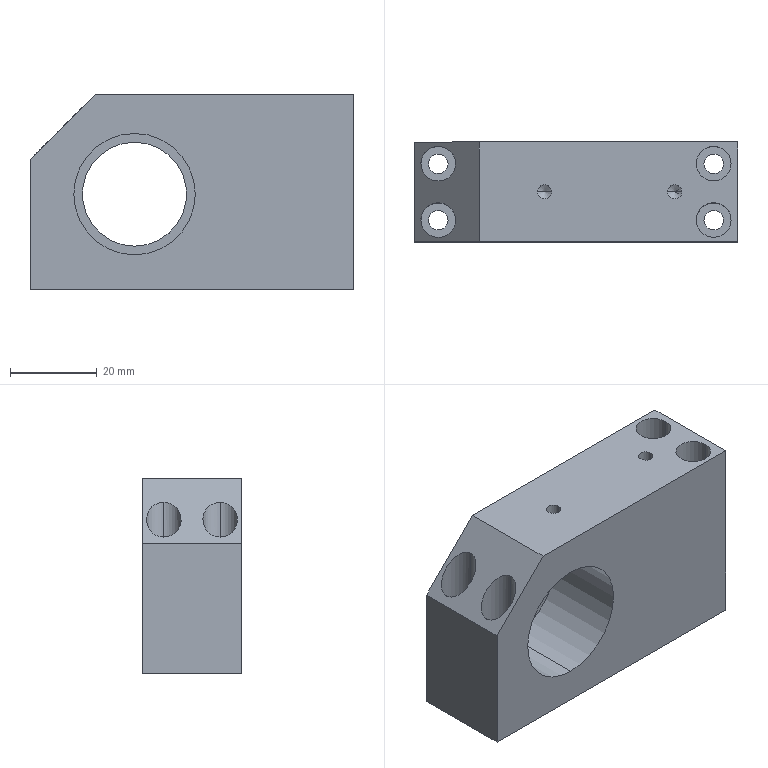Part | SolidWorks | features BaseBody 1 | 1 solid | 40 faces | box 74.5 x 23 x 45 mm | volume 54150 mm3 | cylinder 24 | plane 12 | cone 4 | commonest cylinder face diameters 4.5 x8 8 x8 3.3 x4 24 x2 28 x2
STEP:
#1=CARTESIAN_POINT('',(-13.25,19.,-12.5));
#2=VERTEX_POINT('',#1);
#3=CARTESIAN_POINT('',(-13.25,19.,11.5));
#4=VERTEX_POINT('',#3);
#5=CARTESIAN_POINT('',(-13.25,19.,-0.5));
#6=DIRECTION('',(0.,1.,0.));
#7=DIRECTION('',(0.,0.,1.));
#8=AXIS2_PLACEMENT_3D('',#5,#6,#7);
#9=CIRCLE('',#8,12.);
#10=EDGE_CURVE('',#2,#4,#9,.T.);
#11=ORIENTED_EDGE('',*,*,#10,.F.);
#12=CARTESIAN_POINT('',(-13.25,23.,-12.5));
#13=VERTEX_POINT('',#12);
#14=CARTESIAN_POINT('',(-13.25,-88.,-12.5));
#15=DIRECTION('',(0.,1.,0.));
#16=VECTOR('',#15,1000.);
#17=LINE('',#14,#16);
#18=EDGE_CURVE('',#2,#13,#17,.T.);
#19=ORIENTED_EDGE('',*,*,#18,.T.);
#20=CARTESIAN_POINT('',(-13.25,23.,11.5));
#21=VERTEX_POINT('',#20);
#22=CARTESIAN_POINT('',(-13.25,23.,-0.5));
#23=DIRECTION('',(0.,-1.,0.));
#24=DIRECTION('',(0.,0.,1.));
#25=AXIS2_PLACEMENT_3D('',#22,#23,#24);
#26=CIRCLE('',#25,12.);
#27=EDGE_CURVE('',#21,#13,#26,.T.);
#28=ORIENTED_EDGE('',*,*,#27,.F.);
#29=CARTESIAN_POINT('',(-13.25,-88.,11.5));
#30=DIRECTION('',(0.,1.,0.));
#31=VECTOR('',#30,1000.);
#32=LINE('',#29,#31);
#33=EDGE_CURVE('',#4,#21,#32,.T.);
#34=ORIENTED_EDGE('',*,*,#33,.F.);
#35=EDGE_LOOP('',(#11,#19,#28,#34));
#36=FACE_OUTER_BOUND('',#35,.T.);
#37=CARTESIAN_POINT('',(-13.25,-88.,-0.5));
#38=DIRECTION('',(0.,1.,0.));
#39=DIRECTION('',(0.,0.,1.));
#40=AXIS2_PLACEMENT_3D('',#37,#38,#39);
#41=CYLINDRICAL_SURFACE('',#40,12.);
#42=ADVANCED_FACE('',(#36),#41,.F.);
#43=CARTESIAN_POINT('',(-29.5,5.,-22.5));
#44=VERTEX_POINT('',#43);
#45=CARTESIAN_POINT('',(-34.,5.,-22.5));
#46=VERTEX_POINT('',#45);
#47=CARTESIAN_POINT('',(-31.75,5.,-22.5));
#48=DIRECTION('',(0.,0.,-1.));
#49=DIRECTION('',(1.,0.,0.));
#50=AXIS2_PLACEMENT_3D('',#47,#48,#49);
#51=CIRCLE('',#50,2.25);
#52=EDGE_CURVE('',#44,#46,#51,.T.);
#53=ORIENTED_EDGE('',*,*,#52,.T.);
#54=CARTESIAN_POINT('',(-34.,5.,-12.5));
#55=VERTEX_POINT('',#54);
#56=CARTESIAN_POINT('',(-34.,5.,22.5));
#57=DIRECTION('',(0.,0.,1.));
#58=VECTOR('',#57,1000.);
#59=LINE('',#56,#58);
#60=EDGE_CURVE('',#46,#55,#59,.T.);
#61=ORIENTED_EDGE('',*,*,#60,.T.);
#62=CARTESIAN_POINT('',(-29.5,5.,-12.5));
#63=VERTEX_POINT('',#62);
#64=CARTESIAN_POINT('',(-31.75,5.,-12.5));
#65=DIRECTION('',(0.,0.,-1.));
#66=DIRECTION('',(1.,0.,0.));
#67=AXIS2_PLACEMENT_3D('',#64,#65,#66);
#68=CIRCLE('',#67,2.25);
#69=EDGE_CURVE('',#63,#55,#68,.T.);
#70=ORIENTED_EDGE('',*,*,#69,.F.);
#71=CARTESIAN_POINT('',(-29.5,5.,22.5));
#72=DIRECTION('',(0.,0.,1.));
#73=VECTOR('',#72,1000.);
#74=LINE('',#71,#73);
#75=EDGE_CURVE('',#44,#63,#74,.T.);
#76=ORIENTED_EDGE('',*,*,#75,.F.);
#77=EDGE_LOOP('',(#53,#61,#70,#76));
#78=FACE_OUTER_BOUND('',#77,.T.);
#79=CARTESIAN_POINT('',(-31.75,5.,22.5));
#80=DIRECTION('',(0.,0.,1.));
#81=DIRECTION('',(1.,0.,0.));
#82=AXIS2_PLACEMENT_3D('',#79,#80,#81);
#83=CYLINDRICAL_SURFACE('',#82,2.25);
#84=ADVANCED_FACE('',(#78),#83,.F.);
#85=CARTESIAN_POINT('',(34.,5.,-22.5));
#86=VERTEX_POINT('',#85);
#87=CARTESIAN_POINT('',(29.5,5.,-22.5));
#88=VERTEX_POINT('',#87);
#89=CARTESIAN_POINT('',(31.75,5.,-22.5));
#90=DIRECTION('',(0.,0.,-1.));
#91=DIRECTION('',(1.,0.,0.));
#92=AXIS2_PLACEMENT_3D('',#89,#90,#91);
#93=CIRCLE('',#92,2.25);
#94=EDGE_CURVE('',#86,#88,#93,.T.);
#95=ORIENTED_EDGE('',*,*,#94,.T.);
#96=CARTESIAN_POINT('',(29.5,5.,-12.5));
#97=VERTEX_POINT('',#96);
#98=CARTESIAN_POINT('',(29.5,5.,22.5));
#99=DIRECTION('',(0.,0.,1.));
#100=VECTOR('',#99,1000.);
#101=LINE('',#98,#100);
#102=EDGE_CURVE('',#88,#97,#101,.T.);
#103=ORIENTED_EDGE('',*,*,#102,.T.);
#104=CARTESIAN_POINT('',(34.,5.,-12.5));
#105=VERTEX_POINT('',#104);
#106=CARTESIAN_POINT('',(31.75,5.,-12.5));
#107=DIRECTION('',(0.,0.,-1.));
#108=DIRECTION('',(1.,0.,0.));
#109=AXIS2_PLACEMENT_3D('',#106,#107,#108);
#110=CIRCLE('',#109,2.25);
#111=EDGE_CURVE('',#105,#97,#110,.T.);
#112=ORIENTED_EDGE('',*,*,#111,.F.);
#113=CARTESIAN_POINT('',(34.,5.,22.5));
#114=DIRECTION('',(0.,0.,1.));
#115=VECTOR('',#114,1000.);
#116=LINE('',#113,#115);
#117=EDGE_CURVE('',#86,#105,#116,.T.);
#118=ORIENTED_EDGE('',*,*,#117,.F.);
#119=EDGE_LOOP('',(#95,#103,#112,#118));
#120=FACE_OUTER_BOUND('',#119,.T.);
#121=CARTESIAN_POINT('',(31.75,5.,22.5));
#122=DIRECTION('',(0.,0.,1.));
#123=DIRECTION('',(1.,0.,0.));
#124=AXIS2_PLACEMENT_3D('',#121,#122,#123);
#125=CYLINDRICAL_SURFACE('',#124,2.25);
#126=ADVANCED_FACE('',(#120),#125,.F.);
#127=CARTESIAN_POINT('',(-29.5,18.,-22.5));
#128=VERTEX_POINT('',#127);
#129=CARTESIAN_POINT('',(-34.,18.,-22.5));
#130=VERTEX_POINT('',#129);
#131=CARTESIAN_POINT('',(-31.75,18.,-22.5));
#132=DIRECTION('',(0.,0.,-1.));
#133=DIRECTION('',(1.,0.,0.));
#134=AXIS2_PLACEMENT_3D('',#131,#132,#133);
#135=CIRCLE('',#134,2.25);
#136=EDGE_CURVE('',#128,#130,#135,.T.);
#137=ORIENTED_EDGE('',*,*,#136,.T.);
#138=CARTESIAN_POINT('',(-34.,18.,-12.5));
#139=VERTEX_POINT('',#138);
#140=CARTESIAN_POINT('',(-34.,18.,22.5));
#141=DIRECTION('',(0.,0.,1.));
#142=VECTOR('',#141,1000.);
#143=LINE('',#140,#142);
#144=EDGE_CURVE('',#130,#139,#143,.T.);
#145=ORIENTED_EDGE('',*,*,#144,.T.);
#146=CARTESIAN_POINT('',(-29.5,18.,-12.5));
#147=VERTEX_POINT('',#146);
#148=CARTESIAN_POINT('',(-31.75,18.,-12.5));
#149=DIRECTION('',(0.,0.,-1.));
#150=DIRECTION('',(1.,0.,0.));
#151=AXIS2_PLACEMENT_3D('',#148,#149,#150);
#152=CIRCLE('',#151,2.25);
#153=EDGE_CURVE('',#147,#139,#152,.T.);
#154=ORIENTED_EDGE('',*,*,#153,.F.);
#155=CARTESIAN_POINT('',(-29.5,18.,22.5));
#156=DIRECTION('',(0.,0.,1.));
#157=VECTOR('',#156,1000.);
#158=LINE('',#155,#157);
#159=EDGE_CURVE('',#128,#147,#158,.T.);
#160=ORIENTED_EDGE('',*,*,#159,.F.);
#161=EDGE_LOOP('',(#137,#145,#154,#160));
#162=FACE_OUTER_BOUND('',#161,.T.);
#163=CARTESIAN_POINT('',(-31.75,18.,22.5));
#164=DIRECTION('',(0.,0.,1.));
#165=DIRECTION('',(1.,0.,0.));
#166=AXIS2_PLACEMENT_3D('',#163,#164,#165);
#167=CYLINDRICAL_SURFACE('',#166,2.25);
#168=ADVANCED_FACE('',(#162),#167,.F.);
#169=CARTESIAN_POINT('',(34.,18.,-22.5));
#170=VERTEX_POINT('',#169);
#171=CARTESIAN_POINT('',(29.5,18.,-22.5));
#172=VERTEX_POINT('',#171);
#173=CARTESIAN_POINT('',(31.75,18.,-22.5));
#174=DIRECTION('',(0.,0.,-1.));
#175=DIRECTION('',(1.,0.,0.));
#176=AXIS2_PLACEMENT_3D('',#173,#174,#175);
#177=CIRCLE('',#176,2.25);
#178=EDGE_CURVE('',#170,#172,#177,.T.);
#179=ORIENTED_EDGE('',*,*,#178,.T.);
#180=CARTESIAN_POINT('',(29.5,18.,-12.5));
#181=VERTEX_POINT('',#180);
#182=CARTESIAN_POINT('',(29.5,18.,22.5));
#183=DIRECTION('',(0.,0.,1.));
#184=VECTOR('',#183,1000.);
#185=LINE('',#182,#184);
#186=EDGE_CURVE('',#172,#181,#185,.T.);
#187=ORIENTED_EDGE('',*,*,#186,.T.);
#188=CARTESIAN_POINT('',(34.,18.,-12.5));
#189=VERTEX_POINT('',#188);
#190=CARTESIAN_POINT('',(31.75,18.,-12.5));
#191=DIRECTION('',(0.,0.,-1.));
#192=DIRECTION('',(1.,0.,0.));
#193=AXIS2_PLACEMENT_3D('',#190,#191,#192);
#194=CIRCLE('',#193,2.25);
#195=EDGE_CURVE('',#189,#181,#194,.T.);
#196=ORIENTED_EDGE('',*,*,#195,.F.);
#197=CARTESIAN_POINT('',(34.,18.,22.5));
#198=DIRECTION('',(0.,0.,1.));
#199=VECTOR('',#198,1000.);
#200=LINE('',#197,#199);
#201=EDGE_CURVE('',#170,#189,#200,.T.);
#202=ORIENTED_EDGE('',*,*,#201,.F.);
#203=EDGE_LOOP('',(#179,#187,#196,#202));
#204=FACE_OUTER_BOUND('',#203,.T.);
#205=CARTESIAN_POINT('',(31.75,18.,22.5));
#206=DIRECTION('',(0.,0.,1.));
#207=DIRECTION('',(1.,0.,0.));
#208=AXIS2_PLACEMENT_3D('',#205,#206,#207);
#209=CYLINDRICAL_SURFACE('',#208,2.25);
#210=ADVANCED_FACE('',(#204),#209,.F.);
#211=CARTESIAN_POINT('',(27.75,5.,-12.5));
#212=VERTEX_POINT('',#211);
#213=CARTESIAN_POINT('',(35.75,5.,-12.5));
#214=VERTEX_POINT('',#213);
#215=CARTESIAN_POINT('',(31.75,5.,-12.5));
#216=DIRECTION('',(0.,0.,1.));
#217=DIRECTION('',(1.,0.,0.));
#218=AXIS2_PLACEMENT_3D('',#215,#216,#217);
#219=CIRCLE('',#218,4.);
#220=EDGE_CURVE('',#212,#214,#219,.T.);
#221=ORIENTED_EDGE('',*,*,#220,.F.);
#222=CARTESIAN_POINT('',(27.75,5.,22.5));
#223=VERTEX_POINT('',#222);
#224=CARTESIAN_POINT('',(27.75,5.,22.5));
#225=DIRECTION('',(0.,0.,1.));
#226=VECTOR('',#225,1000.);
#227=LINE('',#224,#226);
#228=EDGE_CURVE('',#212,#223,#227,.T.);
#229=ORIENTED_EDGE('',*,*,#228,.T.);
#230=CARTESIAN_POINT('',(35.75,5.,22.5));
#231=VERTEX_POINT('',#230);
#232=CARTESIAN_POINT('',(31.75,5.,22.5));
#233=DIRECTION('',(0.,0.,1.));
#234=DIRECTION('',(1.,0.,0.));
#235=AXIS2_PLACEMENT_3D('',#232,#233,#234);
#236=CIRCLE('',#235,4.);
#237=EDGE_CURVE('',#223,#231,#236,.T.);
#238=ORIENTED_EDGE('',*,*,#237,.T.);
#239=CARTESIAN_POINT('',(35.75,5.,22.5));
#240=DIRECTION('',(0.,0.,1.));
#241=VECTOR('',#240,1000.);
#242=LINE('',#239,#241);
#243=EDGE_CURVE('',#214,#231,#242,.T.);
#244=ORIENTED_EDGE('',*,*,#243,.F.);
#245=EDGE_LOOP('',(#221,#229,#238,#244));
#246=FACE_OUTER_BOUND('',#245,.T.);
#247=CARTESIAN_POINT('',(31.75,5.,22.5));
#248=DIRECTION('',(0.,0.,1.));
#249=DIRECTION('',(1.,0.,0.));
#250=AXIS2_PLACEMENT_3D('',#247,#248,#249);
#251=CYLINDRICAL_SURFACE('',#250,4.);
#252=ADVANCED_FACE('',(#246),#251,.F.);
#253=CARTESIAN_POINT('',(27.75,18.,-12.5));
#254=VERTEX_POINT('',#253);
#255=CARTESIAN_POINT('',(35.75,18.,-12.5));
#256=VERTEX_POINT('',#255);
#257=CARTESIAN_POINT('',(31.75,18.,-12.5));
#258=DIRECTION('',(0.,0.,1.));
#259=DIRECTION('',(1.,0.,0.));
#260=AXIS2_PLACEMENT_3D('',#257,#258,#259);
#261=CIRCLE('',#260,4.);
#262=EDGE_CURVE('',#254,#256,#261,.T.);
#263=ORIENTED_EDGE('',*,*,#262,.F.);
#264=CARTESIAN_POINT('',(27.75,18.,22.5));
#265=VERTEX_POINT('',#264);
#266=CARTESIAN_POINT('',(27.75,18.,22.5));
#267=DIRECTION('',(0.,0.,1.));
#268=VECTOR('',#267,1000.);
#269=LINE('',#266,#268);
#270=EDGE_CURVE('',#254,#265,#269,.T.);
#271=ORIENTED_EDGE('',*,*,#270,.T.);
#272=CARTESIAN_POINT('',(35.75,18.,22.5));
#273=VERTEX_POINT('',#272);
#274=CARTESIAN_POINT('',(31.75,18.,22.5));
#275=DIRECTION('',(0.,0.,1.));
#276=DIRECTION('',(1.,0.,0.));
#277=AXIS2_PLACEMENT_3D('',#274,#275,#276);
#278=CIRCLE('',#277,4.);
#279=EDGE_CURVE('',#265,#273,#278,.T.);
#280=ORIENTED_EDGE('',*,*,#279,.T.);
#281=CARTESIAN_POINT('',(35.75,18.,22.5));
#282=DIRECTION('',(0.,0.,1.));
#283=VECTOR('',#282,1000.);
#284=LINE('',#281,#283);
#285=EDGE_CURVE('',#256,#273,#284,.T.);
#286=ORIENTED_EDGE('',*,*,#285,.F.);
#287=EDGE_LOOP('',(#263,#271,#280,#286));
#288=FACE_OUTER_BOUND('',#287,.T.);
#289=CARTESIAN_POINT('',(31.75,18.,22.5));
#290=DIRECTION('',(0.,0.,1.));
#291=DIRECTION('',(1.,0.,0.));
#292=AXIS2_PLACEMENT_3D('',#289,#290,#291);
#293=CYLINDRICAL_SURFACE('',#292,4.);
#294=ADVANCED_FACE('',(#288),#293,.F.);
#295=CARTESIAN_POINT('',(-8.9,11.5,14.5));
#296=VERTEX_POINT('',#295);
#297=CARTESIAN_POINT('',(-5.6,11.5,14.5));
#298=VERTEX_POINT('',#297);
#299=CARTESIAN_POINT('',(-7.25,11.5,14.5));
#300=DIRECTION('',(0.,0.,1.));
#301=DIRECTION('',(1.,0.,0.));
#302=AXIS2_PLACEMENT_3D('',#299,#300,#301);
#303=CIRCLE('',#302,1.65);
#304=EDGE_CURVE('',#296,#298,#303,.T.);
#305=ORIENTED_EDGE('',*,*,#304,.F.);
#306=CARTESIAN_POINT('',(-8.9,11.5,22.5));
#307=VERTEX_POINT('',#306);
#308=CARTESIAN_POINT('',(-8.9,11.5,22.5));
#309=DIRECTION('',(0.,0.,1.));
#310=VECTOR('',#309,1000.);
#311=LINE('',#308,#310);
#312=EDGE_CURVE('',#296,#307,#311,.T.);
#313=ORIENTED_EDGE('',*,*,#312,.T.);
#314=CARTESIAN_POINT('',(-5.6,11.5,22.5));
#315=VERTEX_POINT('',#314);
#316=CARTESIAN_POINT('',(-7.25,11.5,22.5));
#317=DIRECTION('',(0.,0.,1.));
#318=DIRECTION('',(1.,0.,0.));
#319=AXIS2_PLACEMENT_3D('',#316,#317,#318);
#320=CIRCLE('',#319,1.65);
#321=EDGE_CURVE('',#307,#315,#320,.T.);
#322=ORIENTED_EDGE('',*,*,#321,.T.);
#323=CARTESIAN_POINT('',(-5.6,11.5,22.5));
#324=DIRECTION('',(0.,0.,1.));
#325=VECTOR('',#324,1000.);
#326=LINE('',#323,#325);
#327=EDGE_CURVE('',#298,#315,#326,.T.);
#328=ORIENTED_EDGE('',*,*,#327,.F.);
#329=EDGE_LOOP('',(#305,#313,#322,#328));
#330=FACE_OUTER_BOUND('',#329,.T.);
#331=CARTESIAN_POINT('',(-7.25,11.5,22.5));
#332=DIRECTION('',(0.,0.,1.));
#333=DIRECTION('',(1.,0.,0.));
#334=AXIS2_PLACEMENT_3D('',#331,#332,#333);
#335=CYLINDRICAL_SURFACE('',#334,1.65);
#336=ADVANCED_FACE('',(#330),#335,.F.);
#337=CARTESIAN_POINT('',(21.1,11.5,14.5));
#338=VERTEX_POINT('',#337);
#339=CARTESIAN_POINT('',(24.4,11.5,14.5));
#340=VERTEX_POINT('',#339);
#341=CARTESIAN_POINT('',(22.75,11.5,14.5));
#342=DIRECTION('',(0.,0.,1.));
#343=DIRECTION('',(1.,0.,0.));
#344=AXIS2_PLACEMENT_3D('',#341,#342,#343);
#345=CIRCLE('',#344,1.65);
#346=EDGE_CURVE('',#338,#340,#345,.T.);
#347=ORIENTED_EDGE('',*,*,#346,.F.);
#348=CARTESIAN_POINT('',(21.1,11.5,22.5));
#349=VERTEX_POINT('',#348);
#350=CARTESIAN_POINT('',(21.1,11.5,22.5));
#351=DIRECTION('',(0.,0.,1.));
#352=VECTOR('',#351,1000.);
#353=LINE('',#350,#352);
#354=EDGE_CURVE('',#338,#349,#353,.T.);
#355=ORIENTED_EDGE('',*,*,#354,.T.);
#356=CARTESIAN_POINT('',(24.4,11.5,22.5));
#357=VERTEX_POINT('',#356);
#358=CARTESIAN_POINT('',(22.75,11.5,22.5));
#359=DIRECTION('',(0.,0.,1.));
#360=DIRECTION('',(1.,0.,0.));
#361=AXIS2_PLACEMENT_3D('',#358,#359,#360);
#362=CIRCLE('',#361,1.65);
#363=EDGE_CURVE('',#349,#357,#362,.T.);
#364=ORIENTED_EDGE('',*,*,#363,.T.);
#365=CARTESIAN_POINT('',(24.4,11.5,22.5));
#366=DIRECTION('',(0.,0.,1.));
#367=VECTOR('',#366,1000.);
#368=LINE('',#365,#367);
#369=EDGE_CURVE('',#340,#357,#368,.T.);
#370=ORIENTED_EDGE('',*,*,#369,.F.);
#371=EDGE_LOOP('',(#347,#355,#364,#370));
#372=FACE_OUTER_BOUND('',#371,.T.);
#373=CARTESIAN_POINT('',(22.75,11.5,22.5));
#374=DIRECTION('',(0.,0.,1.));
#375=DIRECTION('',(1.,0.,0.));
#376=AXIS2_PLACEMENT_3D('',#373,#374,#375);
#377=CYLINDRICAL_SURFACE('',#376,1.65);
#378=ADVANCED_FACE('',(#372),#377,.F.);
#379=CARTESIAN_POINT('',(-35.75,5.,-12.5));
#380=VERTEX_POINT('',#379);
#381=CARTESIAN_POINT('',(-27.75,5.,-12.5));
#382=VERTEX_POINT('',#381);
#383=CARTESIAN_POINT('',(-31.75,5.,-12.5));
#384=DIRECTION('',(0.,0.,1.));
#385=DIRECTION('',(1.,0.,0.));
#386=AXIS2_PLACEMENT_3D('',#383,#384,#385);
#387=CIRCLE('',#386,4.);
#388=EDGE_CURVE('',#380,#382,#387,.T.);
#389=ORIENTED_EDGE('',*,*,#388,.F.);
#390=CARTESIAN_POINT('',(-35.75,5.,9.));
#391=VERTEX_POINT('',#390);
#392=CARTESIAN_POINT('',(-35.75,5.,22.5));
#393=DIRECTION('',(0.,0.,1.));
#394=VECTOR('',#393,1000.);
#395=LINE('',#392,#394);
#396=EDGE_CURVE('',#380,#391,#395,.T.);
#397=ORIENTED_EDGE('',*,*,#396,.T.);
#398=CARTESIAN_POINT('',(-27.75,5.,17.));
#399=VERTEX_POINT('',#398);
#400=CARTESIAN_POINT('',(-35.75,5.,9.));
#401=CARTESIAN_POINT('',(-35.75,-3.,9.));
#402=CARTESIAN_POINT('',(-27.75,-3.,17.));
#403=CARTESIAN_POINT('',(-27.75,5.,17.));
#404=(BOUNDED_CURVE()B_SPLINE_CURVE(3,(#400,#401,#402,#403),.UNSPECIFIED.,.F.,.F.)B_SPLINE_CURVE_WITH_KNOTS((4,4),(3.142,6.283),.UNSPECIFIED.)CURVE()GEOMETRIC_REPRESENTATION_ITEM()RATIONAL_B_SPLINE_CURVE((1.,0.3333,0.3333,1.))REPRESENTATION_ITEM(''));
#405=EDGE_CURVE('',#391,#399,#404,.T.);
#406=ORIENTED_EDGE('',*,*,#405,.T.);
#407=CARTESIAN_POINT('',(-27.75,5.,22.5));
#408=DIRECTION('',(0.,0.,1.));
#409=VECTOR('',#408,1000.);
#410=LINE('',#407,#409);
#411=EDGE_CURVE('',#382,#399,#410,.T.);
#412=ORIENTED_EDGE('',*,*,#411,.F.);
#413=EDGE_LOOP('',(#389,#397,#406,#412));
#414=FACE_OUTER_BOUND('',#413,.T.);
#415=CARTESIAN_POINT('',(-31.75,5.,22.5));
#416=DIRECTION('',(0.,0.,1.));
#417=DIRECTION('',(1.,0.,0.));
#418=AXIS2_PLACEMENT_3D('',#415,#416,#417);
#419=CYLINDRICAL_SURFACE('',#418,4.);
#420=ADVANCED_FACE('',(#414),#419,.F.);
#421=CARTESIAN_POINT('',(-35.75,18.,-12.5));
#422=VERTEX_POINT('',#421);
#423=CARTESIAN_POINT('',(-27.75,18.,-12.5));
#424=VERTEX_POINT('',#423);
#425=CARTESIAN_POINT('',(-31.75,18.,-12.5));
#426=DIRECTION('',(0.,0.,1.));
#427=DIRECTION('',(1.,0.,0.));
#428=AXIS2_PLACEMENT_3D('',#425,#426,#427);
#429=CIRCLE('',#428,4.);
#430=EDGE_CURVE('',#422,#424,#429,.T.);
#431=ORIENTED_EDGE('',*,*,#430,.F.);
#432=CARTESIAN_POINT('',(-35.75,18.,9.));
#433=VERTEX_POINT('',#432);
#434=CARTESIAN_POINT('',(-35.75,18.,22.5));
#435=DIRECTION('',(0.,0.,1.));
#436=VECTOR('',#435,1000.);
#437=LINE('',#434,#436);
#438=EDGE_CURVE('',#422,#433,#437,.T.);
#439=ORIENTED_EDGE('',*,*,#438,.T.);
#440=CARTESIAN_POINT('',(-27.75,18.,17.));
#441=VERTEX_POINT('',#440);
#442=CARTESIAN_POINT('',(-35.75,18.,9.));
#443=CARTESIAN_POINT('',(-35.75,10.,9.));
#444=CARTESIAN_POINT('',(-27.75,10.,17.));
#445=CARTESIAN_POINT('',(-27.75,18.,17.));
#446=(BOUNDED_CURVE()B_SPLINE_CURVE(3,(#442,#443,#444,#445),.UNSPECIFIED.,.F.,.F.)B_SPLINE_CURVE_WITH_KNOTS((4,4),(3.142,6.283),.UNSPECIFIED.)CURVE()GEOMETRIC_REPRESENTATION_ITEM()RATIONAL_B_SPLINE_CURVE((1.,0.3333,0.3333,1.))REPRESENTATION_ITEM(''));
#447=EDGE_CURVE('',#433,#441,#446,.T.);
#448=ORIENTED_EDGE('',*,*,#447,.T.);
#449=CARTESIAN_POINT('',(-27.75,18.,22.5));
#450=DIRECTION('',(0.,0.,1.));
#451=VECTOR('',#450,1000.);
#452=LINE('',#449,#451);
#453=EDGE_CURVE('',#424,#441,#452,.T.);
#454=ORIENTED_EDGE('',*,*,#453,.F.);
#455=EDGE_LOOP('',(#431,#439,#448,#454));
#456=FACE_OUTER_BOUND('',#455,.T.);
#457=CARTESIAN_POINT('',(-31.75,18.,22.5));
#458=DIRECTION('',(0.,0.,1.));
#459=DIRECTION('',(1.,0.,0.));
#460=AXIS2_PLACEMENT_3D('',#457,#458,#459);
#461=CYLINDRICAL_SURFACE('',#460,4.);
#462=ADVANCED_FACE('',(#456),#461,.F.);
#463=CARTESIAN_POINT('',(-13.25,19.,13.5));
#464=VERTEX_POINT('',#463);
#465=CARTESIAN_POINT('',(-13.25,19.,-14.5));
#466=VERTEX_POINT('',#465);
#467=CARTESIAN_POINT('',(-13.25,19.,-0.5));
#468=DIRECTION('',(0.,-1.,0.));
#469=DIRECTION('',(0.,0.,-1.));
#470=AXIS2_PLACEMENT_3D('',#467,#468,#469);
#471=CIRCLE('',#470,14.);
#472=EDGE_CURVE('',#464,#466,#471,.T.);
#473=ORIENTED_EDGE('',*,*,#472,.F.);
#474=CARTESIAN_POINT('',(-13.25,0.,13.5));
#475=VERTEX_POINT('',#474);
#476=CARTESIAN_POINT('',(-13.25,19.,13.5));
#477=DIRECTION('',(0.,-1.,0.));
#478=VECTOR('',#477,1000.);
#479=LINE('',#476,#478);
#480=EDGE_CURVE('',#464,#475,#479,.T.);
#481=ORIENTED_EDGE('',*,*,#480,.T.);
#482=CARTESIAN_POINT('',(-13.25,0.,-14.5));
#483=VERTEX_POINT('',#482);
#484=CARTESIAN_POINT('',(-13.25,0.,-0.5));
#485=DIRECTION('',(0.,-1.,0.));
#486=DIRECTION('',(0.,0.,-1.));
#487=AXIS2_PLACEMENT_3D('',#484,#485,#486);
#488=CIRCLE('',#487,14.);
#489=EDGE_CURVE('',#475,#483,#488,.T.);
#490=ORIENTED_EDGE('',*,*,#489,.T.);
#491=CARTESIAN_POINT('',(-13.25,19.,-14.5));
#492=DIRECTION('',(0.,-1.,0.));
#493=VECTOR('',#492,1000.);
#494=LINE('',#491,#493);
#495=EDGE_CURVE('',#466,#483,#494,.T.);
#496=ORIENTED_EDGE('',*,*,#495,.F.);
#497=EDGE_LOOP('',(#473,#481,#490,#496));
#498=FACE_OUTER_BOUND('',#497,.T.);
#499=CARTESIAN_POINT('',(-13.25,19.,-0.5));
#500=DIRECTION('',(0.,-1.,0.));
#501=DIRECTION('',(0.,0.,-1.));
#502=AXIS2_PLACEMENT_3D('',#499,#500,#501);
#503=CYLINDRICAL_SURFACE('',#502,14.);
#504=ADVANCED_FACE('',(#498),#503,.F.);
#505=CARTESIAN_POINT('',(-7.25,11.5,13.509));
#506=VERTEX_POINT('',#505);
#507=CARTESIAN_POINT('',(-5.6,11.5,14.5));
#508=DIRECTION('',(0.8572,0.,0.515));
#509=VECTOR('',#508,1000.);
#510=LINE('',#507,#509);
#511=EDGE_CURVE('',#506,#298,#510,.T.);
#512=ORIENTED_EDGE('',*,*,#511,.F.);
#513=CARTESIAN_POINT('',(-8.9,11.5,14.5));
#514=DIRECTION('',(-0.8572,0.,0.515));
#515=VECTOR('',#514,1000.);
#516=LINE('',#513,#515);
#517=EDGE_CURVE('',#506,#296,#516,.T.);
#518=ORIENTED_EDGE('',*,*,#517,.T.);
#519=ORIENTED_EDGE('',*,*,#304,.T.);
#520=EDGE_LOOP('',(#512,#518,#519));
#521=FACE_OUTER_BOUND('',#520,.T.);
#522=CARTESIAN_POINT('',(-7.25,11.5,14.5));
#523=DIRECTION('',(0.,0.,1.));
#524=DIRECTION('',(1.,0.,0.));
#525=AXIS2_PLACEMENT_3D('',#522,#523,#524);
#526=CONICAL_SURFACE('',#525,1.65,1.03);
#527=ADVANCED_FACE('',(#521),#526,.F.);
#528=CARTESIAN_POINT('',(22.75,11.5,13.509));
#529=VERTEX_POINT('',#528);
#530=CARTESIAN_POINT('',(24.4,11.5,14.5));
#531=DIRECTION('',(0.8572,0.,0.515));
#532=VECTOR('',#531,1000.);
#533=LINE('',#530,#532);
#534=EDGE_CURVE('',#529,#340,#533,.T.);
#535=ORIENTED_EDGE('',*,*,#534,.F.);
#536=CARTESIAN_POINT('',(21.1,11.5,14.5));
#537=DIRECTION('',(-0.8572,0.,0.515));
#538=VECTOR('',#537,1000.);
#539=LINE('',#536,#538);
#540=EDGE_CURVE('',#529,#338,#539,.T.);
#541=ORIENTED_EDGE('',*,*,#540,.T.);
#542=ORIENTED_EDGE('',*,*,#346,.T.);
#543=EDGE_LOOP('',(#535,#541,#542));
#544=FACE_OUTER_BOUND('',#543,.T.);
#545=CARTESIAN_POINT('',(22.75,11.5,14.5));
#546=DIRECTION('',(0.,0.,1.));
#547=DIRECTION('',(1.,0.,0.));
#548=AXIS2_PLACEMENT_3D('',#545,#546,#547);
#549=CONICAL_SURFACE('',#548,1.65,1.03);
#550=ADVANCED_FACE('',(#544),#549,.F.);
#551=ORIENTED_EDGE('',*,*,#27,.T.);
#552=CARTESIAN_POINT('',(-13.25,23.,-0.5));
#553=DIRECTION('',(0.,-1.,0.));
#554=DIRECTION('',(0.,0.,1.));
#555=AXIS2_PLACEMENT_3D('',#552,#553,#554);
#556=CIRCLE('',#555,12.);
#557=EDGE_CURVE('',#13,#21,#556,.T.);
#558=ORIENTED_EDGE('',*,*,#557,.T.);
#559=EDGE_LOOP('',(#551,#558));
#560=FACE_BOUND('',#559,.T.);
#561=CARTESIAN_POINT('',(37.25,23.,-22.5));
#562=VERTEX_POINT('',#561);
#563=CARTESIAN_POINT('',(-37.25,23.,-22.5));
#564=VERTEX_POINT('',#563);
#565=CARTESIAN_POINT('',(0.,23.,-22.5));
#566=DIRECTION('',(-1.,0.,0.));
#567=VECTOR('',#566,1000.);
#568=LINE('',#565,#567);
#569=EDGE_CURVE('',#562,#564,#568,.T.);
#570=ORIENTED_EDGE('',*,*,#569,.T.);
#571=CARTESIAN_POINT('',(-37.25,23.,7.5));
#572=VERTEX_POINT('',#571);
#573=CARTESIAN_POINT('',(-37.25,23.,0.));
#574=DIRECTION('',(0.,0.,1.));
#575=VECTOR('',#574,1000.);
#576=LINE('',#573,#575);
#577=EDGE_CURVE('',#564,#572,#576,.T.);
#578=ORIENTED_EDGE('',*,*,#577,.T.);
#579=CARTESIAN_POINT('',(-22.25,23.,22.5));
#580=VERTEX_POINT('',#579);
#581=CARTESIAN_POINT('',(-37.25,23.,7.5));
#582=DIRECTION('',(0.7071,0.,0.7071));
#583=VECTOR('',#582,1000.);
#584=LINE('',#581,#583);
#585=EDGE_CURVE('',#572,#580,#584,.T.);
#586=ORIENTED_EDGE('',*,*,#585,.T.);
#587=CARTESIAN_POINT('',(37.25,23.,22.5));
#588=VERTEX_POINT('',#587);
#589=CARTESIAN_POINT('',(0.,23.,22.5));
#590=DIRECTION('',(1.,0.,0.));
#591=VECTOR('',#590,1000.);
#592=LINE('',#589,#591);
#593=EDGE_CURVE('',#580,#588,#592,.T.);
#594=ORIENTED_EDGE('',*,*,#593,.T.);
#595=CARTESIAN_POINT('',(37.25,23.,0.));
#596=DIRECTION('',(0.,0.,-1.));
#597=VECTOR('',#596,1000.);
#598=LINE('',#595,#597);
#599=EDGE_CURVE('',#588,#562,#598,.T.);
#600=ORIENTED_EDGE('',*,*,#599,.T.);
#601=EDGE_LOOP('',(#570,#578,#586,#594,#600));
#602=FACE_OUTER_BOUND('',#601,.T.);
#603=CARTESIAN_POINT('',(0.,23.,0.));
#604=DIRECTION('',(0.,1.,0.));
#605=DIRECTION('',(0.,0.,1.));
#606=AXIS2_PLACEMENT_3D('',#603,#604,#605);
#607=PLANE('',#606);
#608=ADVANCED_FACE('',(#560,#602),#607,.T.);
#609=ORIENTED_EDGE('',*,*,#18,.F.);
#610=CARTESIAN_POINT('',(-13.25,19.,-0.5));
#611=DIRECTION('',(0.,1.,0.));
#612=DIRECTION('',(0.,0.,1.));
#613=AXIS2_PLACEMENT_3D('',#610,#611,#612);
#614=CIRCLE('',#613,12.);
#615=EDGE_CURVE('',#4,#2,#614,.T.);
#616=ORIENTED_EDGE('',*,*,#615,.F.);
#617=ORIENTED_EDGE('',*,*,#33,.T.);
#618=ORIENTED_EDGE('',*,*,#557,.F.);
#619=EDGE_LOOP('',(#609,#616,#617,#618));
#620=FACE_OUTER_BOUND('',#619,.T.);
#621=CARTESIAN_POINT('',(-13.25,-88.,-0.5));
#622=DIRECTION('',(0.,1.,0.));
#623=DIRECTION('',(0.,0.,1.));
#624=AXIS2_PLACEMENT_3D('',#621,#622,#623);
#625=CYLINDRICAL_SURFACE('',#624,12.);
#626=ADVANCED_FACE('',(#620),#625,.F.);
#627=CARTESIAN_POINT('',(-37.25,0.,7.5));
#628=VERTEX_POINT('',#627);
#629=CARTESIAN_POINT('',(-37.25,23.,7.5));
#630=DIRECTION('',(0.,-1.,0.));
#631=VECTOR('',#630,1000.);
#632=LINE('',#629,#631);
#633=EDGE_CURVE('',#572,#628,#632,.T.);
#634=ORIENTED_EDGE('',*,*,#633,.F.);
#635=ORIENTED_EDGE('',*,*,#577,.F.);
#636=CARTESIAN_POINT('',(-37.25,0.,-22.5));
#637=VERTEX_POINT('',#636);
#638=CARTESIAN_POINT('',(-37.25,23.,-22.5));
#639=DIRECTION('',(0.,1.,0.));
#640=VECTOR('',#639,1000.);
#641=LINE('',#638,#640);
#642=EDGE_CURVE('',#637,#564,#641,.T.);
#643=ORIENTED_EDGE('',*,*,#642,.F.);
#644=CARTESIAN_POINT('',(-37.25,0.,22.5));
#645=DIRECTION('',(0.,0.,-1.));
#646=VECTOR('',#645,1000.);
#647=LINE('',#644,#646);
#648=EDGE_CURVE('',#628,#637,#647,.T.);
#649=ORIENTED_EDGE('',*,*,#648,.F.);
#650=EDGE_LOOP('',(#634,#635,#643,#649));
#651=FACE_OUTER_BOUND('',#650,.T.);
#652=CARTESIAN_POINT('',(-37.25,23.,22.5));
#653=DIRECTION('',(1.,0.,0.));
#654=DIRECTION('',(0.,0.,-1.));
#655=AXIS2_PLACEMENT_3D('',#652,#653,#654);
#656=PLANE('',#655);
#657=ADVANCED_FACE('',(#651),#656,.F.);
#658=ORIENTED_EDGE('',*,*,#642,.T.);
#659=ORIENTED_EDGE('',*,*,#569,.F.);
#660=CARTESIAN_POINT('',(37.25,0.,-22.5));
#661=VERTEX_POINT('',#660);
#662=CARTESIAN_POINT('',(37.25,23.,-22.5));
#663=DIRECTION('',(0.,1.,0.));
#664=VECTOR('',#663,1000.);
#665=LINE('',#662,#664);
#666=EDGE_CURVE('',#661,#562,#665,.T.);
#667=ORIENTED_EDGE('',*,*,#666,.F.);
#668=CARTESIAN_POINT('',(37.25,0.,-22.5));
#669=DIRECTION('',(1.,0.,0.));
#670=VECTOR('',#669,1000.);
#671=LINE('',#668,#670);
#672=EDGE_CURVE('',#637,#661,#671,.T.);
#673=ORIENTED_EDGE('',*,*,#672,.F.);
#674=EDGE_LOOP('',(#658,#659,#667,#673));
#675=FACE_OUTER_BOUND('',#674,.T.);
#676=ORIENTED_EDGE('',*,*,#52,.F.);
#677=CARTESIAN_POINT('',(-31.75,5.,-22.5));
#678=DIRECTION('',(0.,0.,-1.));
#679=DIRECTION('',(1.,0.,0.));
#680=AXIS2_PLACEMENT_3D('',#677,#678,#679);
#681=CIRCLE('',#680,2.25);
#682=EDGE_CURVE('',#46,#44,#681,.T.);
#683=ORIENTED_EDGE('',*,*,#682,.F.);
#684=EDGE_LOOP('',(#676,#683));
#685=FACE_BOUND('',#684,.T.);
#686=ORIENTED_EDGE('',*,*,#94,.F.);
#687=CARTESIAN_POINT('',(31.75,5.,-22.5));
#688=DIRECTION('',(0.,0.,-1.));
#689=DIRECTION('',(1.,0.,0.));
#690=AXIS2_PLACEMENT_3D('',#687,#688,#689);
#691=CIRCLE('',#690,2.25);
#692=EDGE_CURVE('',#88,#86,#691,.T.);
#693=ORIENTED_EDGE('',*,*,#692,.F.);
#694=EDGE_LOOP('',(#686,#693));
#695=FACE_BOUND('',#694,.T.);
#696=ORIENTED_EDGE('',*,*,#136,.F.);
#697=CARTESIAN_POINT('',(-31.75,18.,-22.5));
#698=DIRECTION('',(0.,0.,-1.));
#699=DIRECTION('',(1.,0.,0.));
#700=AXIS2_PLACEMENT_3D('',#697,#698,#699);
#701=CIRCLE('',#700,2.25);
#702=EDGE_CURVE('',#130,#128,#701,.T.);
#703=ORIENTED_EDGE('',*,*,#702,.F.);
#704=EDGE_LOOP('',(#696,#703));
#705=FACE_BOUND('',#704,.T.);
#706=ORIENTED_EDGE('',*,*,#178,.F.);
#707=CARTESIAN_POINT('',(31.75,18.,-22.5));
#708=DIRECTION('',(0.,0.,-1.));
#709=DIRECTION('',(1.,0.,0.));
#710=AXIS2_PLACEMENT_3D('',#707,#708,#709);
#711=CIRCLE('',#710,2.25);
#712=EDGE_CURVE('',#172,#170,#711,.T.);
#713=ORIENTED_EDGE('',*,*,#712,.F.);
#714=EDGE_LOOP('',(#706,#713));
#715=FACE_BOUND('',#714,.T.);
#716=CARTESIAN_POINT('',(37.25,23.,-22.5));
#717=DIRECTION('',(0.,0.,1.));
#718=DIRECTION('',(1.,0.,0.));
#719=AXIS2_PLACEMENT_3D('',#716,#717,#718);
#720=PLANE('',#719);
#721=ADVANCED_FACE('',(#675,#685,#695,#705,#715),#720,.F.);
#722=ORIENTED_EDGE('',*,*,#666,.T.);
#723=ORIENTED_EDGE('',*,*,#599,.F.);
#724=CARTESIAN_POINT('',(37.25,0.,22.5));
#725=VERTEX_POINT('',#724);
#726=CARTESIAN_POINT('',(37.25,23.,22.5));
#727=DIRECTION('',(0.,1.,0.));
#728=VECTOR('',#727,1000.);
#729=LINE('',#726,#728);
#730=EDGE_CURVE('',#725,#588,#729,.T.);
#731=ORIENTED_EDGE('',*,*,#730,.F.);
#732=CARTESIAN_POINT('',(37.25,0.,22.5));
#733=DIRECTION('',(0.,0.,1.));
#734=VECTOR('',#733,1000.);
#735=LINE('',#732,#734);
#736=EDGE_CURVE('',#661,#725,#735,.T.);
#737=ORIENTED_EDGE('',*,*,#736,.F.);
#738=EDGE_LOOP('',(#722,#723,#731,#737));
#739=FACE_OUTER_BOUND('',#738,.T.);
#740=CARTESIAN_POINT('',(37.25,23.,22.5));
#741=DIRECTION('',(-1.,0.,0.));
#742=DIRECTION('',(0.,0.,1.));
#743=AXIS2_PLACEMENT_3D('',#740,#741,#742);
#744=PLANE('',#743);
#745=ADVANCED_FACE('',(#739),#744,.F.);
#746=CARTESIAN_POINT('',(-22.25,0.,22.5));
#747=VERTEX_POINT('',#746);
#748=CARTESIAN_POINT('',(-22.25,23.,22.5));
#749=DIRECTION('',(0.,1.,0.));
#750=VECTOR('',#749,1000.);
#751=LINE('',#748,#750);
#752=EDGE_CURVE('',#747,#580,#751,.T.);
#753=ORIENTED_EDGE('',*,*,#752,.F.);
#754=CARTESIAN_POINT('',(37.25,0.,22.5));
#755=DIRECTION('',(-1.,0.,0.));
#756=VECTOR('',#755,1000.);
#757=LINE('',#754,#756);
#758=EDGE_CURVE('',#725,#747,#757,.T.);
#759=ORIENTED_EDGE('',*,*,#758,.F.);
#760=ORIENTED_EDGE('',*,*,#730,.T.);
#761=ORIENTED_EDGE('',*,*,#593,.F.);
#762=EDGE_LOOP('',(#753,#759,#760,#761));
#763=FACE_OUTER_BOUND('',#762,.T.);
#764=CARTESIAN_POINT('',(31.75,5.,22.5));
#765=DIRECTION('',(0.,0.,1.));
#766=DIRECTION('',(1.,0.,0.));
#767=AXIS2_PLACEMENT_3D('',#764,#765,#766);
#768=CIRCLE('',#767,4.);
#769=EDGE_CURVE('',#231,#223,#768,.T.);
#770=ORIENTED_EDGE('',*,*,#769,.F.);
#771=ORIENTED_EDGE('',*,*,#237,.F.);
#772=EDGE_LOOP('',(#770,#771));
#773=FACE_BOUND('',#772,.T.);
#774=CARTESIAN_POINT('',(31.75,18.,22.5));
#775=DIRECTION('',(0.,0.,1.));
#776=DIRECTION('',(1.,0.,0.));
#777=AXIS2_PLACEMENT_3D('',#774,#775,#776);
#778=CIRCLE('',#777,4.);
#779=EDGE_CURVE('',#273,#265,#778,.T.);
#780=ORIENTED_EDGE('',*,*,#779,.F.);
#781=ORIENTED_EDGE('',*,*,#279,.F.);
#782=EDGE_LOOP('',(#780,#781));
#783=FACE_BOUND('',#782,.T.);
#784=CARTESIAN_POINT('',(-7.25,11.5,22.5));
#785=DIRECTION('',(0.,0.,1.));
#786=DIRECTION('',(1.,0.,0.));
#787=AXIS2_PLACEMENT_3D('',#784,#785,#786);
#788=CIRCLE('',#787,1.65);
#789=EDGE_CURVE('',#315,#307,#788,.T.);
#790=ORIENTED_EDGE('',*,*,#789,.F.);
#791=ORIENTED_EDGE('',*,*,#321,.F.);
#792=EDGE_LOOP('',(#790,#791));
#793=FACE_BOUND('',#792,.T.);
#794=CARTESIAN_POINT('',(22.75,11.5,22.5));
#795=DIRECTION('',(0.,0.,1.));
#796=DIRECTION('',(1.,0.,0.));
#797=AXIS2_PLACEMENT_3D('',#794,#795,#796);
#798=CIRCLE('',#797,1.65);
#799=EDGE_CURVE('',#357,#349,#798,.T.);
#800=ORIENTED_EDGE('',*,*,#799,.F.);
#801=ORIENTED_EDGE('',*,*,#363,.F.);
#802=EDGE_LOOP('',(#800,#801));
#803=FACE_BOUND('',#802,.T.);
#804=CARTESIAN_POINT('',(37.25,23.,22.5));
#805=DIRECTION('',(0.,0.,-1.));
#806=DIRECTION('',(-1.,0.,0.));
#807=AXIS2_PLACEMENT_3D('',#804,#805,#806);
#808=PLANE('',#807);
#809=ADVANCED_FACE('',(#763,#773,#783,#793,#803),#808,.F.);
#810=ORIENTED_EDGE('',*,*,#633,.T.);
#811=CARTESIAN_POINT('',(-22.25,0.,22.5));
#812=DIRECTION('',(-0.7071,0.,-0.7071));
#813=VECTOR('',#812,1000.);
#814=LINE('',#811,#813);
#815=EDGE_CURVE('',#747,#628,#814,.T.);
#816=ORIENTED_EDGE('',*,*,#815,.F.);
#817=ORIENTED_EDGE('',*,*,#752,.T.);
#818=ORIENTED_EDGE('',*,*,#585,.F.);
#819=EDGE_LOOP('',(#810,#816,#817,#818));
#820=FACE_OUTER_BOUND('',#819,.T.);
#821=CARTESIAN_POINT('',(-27.75,5.,17.));
#822=CARTESIAN_POINT('',(-27.75,13.,17.));
#823=CARTESIAN_POINT('',(-35.75,13.,9.));
#824=CARTESIAN_POINT('',(-35.75,5.,9.));
#825=(BOUNDED_CURVE()B_SPLINE_CURVE(3,(#821,#822,#823,#824),.UNSPECIFIED.,.F.,.F.)B_SPLINE_CURVE_WITH_KNOTS((4,4),(0.,3.142),.UNSPECIFIED.)CURVE()GEOMETRIC_REPRESENTATION_ITEM()RATIONAL_B_SPLINE_CURVE((1.,0.3333,0.3333,1.))REPRESENTATION_ITEM(''));
#826=EDGE_CURVE('',#399,#391,#825,.T.);
#827=ORIENTED_EDGE('',*,*,#826,.F.);
#828=ORIENTED_EDGE('',*,*,#405,.F.);
#829=EDGE_LOOP('',(#827,#828));
#830=FACE_BOUND('',#829,.T.);
#831=CARTESIAN_POINT('',(-27.75,18.,17.));
#832=CARTESIAN_POINT('',(-27.75,26.,17.));
#833=CARTESIAN_POINT('',(-35.75,26.,9.));
#834=CARTESIAN_POINT('',(-35.75,18.,9.));
#835=(BOUNDED_CURVE()B_SPLINE_CURVE(3,(#831,#832,#833,#834),.UNSPECIFIED.,.F.,.F.)B_SPLINE_CURVE_WITH_KNOTS((4,4),(0.,3.142),.UNSPECIFIED.)CURVE()GEOMETRIC_REPRESENTATION_ITEM()RATIONAL_B_SPLINE_CURVE((1.,0.3333,0.3333,1.))REPRESENTATION_ITEM(''));
#836=EDGE_CURVE('',#441,#433,#835,.T.);
#837=ORIENTED_EDGE('',*,*,#836,.F.);
#838=ORIENTED_EDGE('',*,*,#447,.F.);
#839=EDGE_LOOP('',(#837,#838));
#840=FACE_BOUND('',#839,.T.);
#841=CARTESIAN_POINT('',(-22.25,35.,22.5));
#842=DIRECTION('',(0.7071,0.,-0.7071));
#843=DIRECTION('',(-0.7071,0.,-0.7071));
#844=AXIS2_PLACEMENT_3D('',#841,#842,#843);
#845=PLANE('',#844);
#846=ADVANCED_FACE('',(#820,#830,#840),#845,.F.);
#847=ORIENTED_EDGE('',*,*,#615,.T.);
#848=ORIENTED_EDGE('',*,*,#10,.T.);
#849=EDGE_LOOP('',(#847,#848));
#850=FACE_BOUND('',#849,.T.);
#851=CARTESIAN_POINT('',(-13.25,19.,-0.5));
#852=DIRECTION('',(0.,-1.,0.));
#853=DIRECTION('',(0.,0.,-1.));
#854=AXIS2_PLACEMENT_3D('',#851,#852,#853);
#855=CIRCLE('',#854,14.);
#856=EDGE_CURVE('',#466,#464,#855,.T.);
#857=ORIENTED_EDGE('',*,*,#856,.T.);
#858=ORIENTED_EDGE('',*,*,#472,.T.);
#859=EDGE_LOOP('',(#857,#858));
#860=FACE_OUTER_BOUND('',#859,.T.);
#861=CARTESIAN_POINT('',(-13.25,19.,-0.5));
#862=DIRECTION('',(0.,-1.,0.));
#863=DIRECTION('',(0.,0.,-1.));
#864=AXIS2_PLACEMENT_3D('',#861,#862,#863);
#865=PLANE('',#864);
#866=ADVANCED_FACE('',(#850,#860),#865,.T.);
#867=ORIENTED_EDGE('',*,*,#815,.T.);
#868=ORIENTED_EDGE('',*,*,#648,.T.);
#869=ORIENTED_EDGE('',*,*,#672,.T.);
#870=ORIENTED_EDGE('',*,*,#736,.T.);
#871=ORIENTED_EDGE('',*,*,#758,.T.);
#872=EDGE_LOOP('',(#867,#868,#869,#870,#871));
#873=FACE_OUTER_BOUND('',#872,.T.);
#874=CARTESIAN_POINT('',(-13.25,0.,-0.5));
#875=DIRECTION('',(0.,-1.,0.));
#876=DIRECTION('',(0.,0.,-1.));
#877=AXIS2_PLACEMENT_3D('',#874,#875,#876);
#878=CIRCLE('',#877,14.);
#879=EDGE_CURVE('',#483,#475,#878,.T.);
#880=ORIENTED_EDGE('',*,*,#879,.F.);
#881=ORIENTED_EDGE('',*,*,#489,.F.);
#882=EDGE_LOOP('',(#880,#881));
#883=FACE_BOUND('',#882,.T.);
#884=CARTESIAN_POINT('',(0.,0.,0.));
#885=DIRECTION('',(0.,1.,0.));
#886=DIRECTION('',(0.,0.,1.));
#887=AXIS2_PLACEMENT_3D('',#884,#885,#886);
#888=PLANE('',#887);
#889=ADVANCED_FACE('',(#873,#883),#888,.F.);
#890=ORIENTED_EDGE('',*,*,#60,.F.);
#891=ORIENTED_EDGE('',*,*,#682,.T.);
#892=ORIENTED_EDGE('',*,*,#75,.T.);
#893=CARTESIAN_POINT('',(-31.75,5.,-12.5));
#894=DIRECTION('',(0.,0.,-1.));
#895=DIRECTION('',(1.,0.,0.));
#896=AXIS2_PLACEMENT_3D('',#893,#894,#895);
#897=CIRCLE('',#896,2.25);
#898=EDGE_CURVE('',#55,#63,#897,.T.);
#899=ORIENTED_EDGE('',*,*,#898,.F.);
#900=EDGE_LOOP('',(#890,#891,#892,#899));
#901=FACE_OUTER_BOUND('',#900,.T.);
#902=CARTESIAN_POINT('',(-31.75,5.,22.5));
#903=DIRECTION('',(0.,0.,1.));
#904=DIRECTION('',(1.,0.,0.));
#905=AXIS2_PLACEMENT_3D('',#902,#903,#904);
#906=CYLINDRICAL_SURFACE('',#905,2.25);
#907=ADVANCED_FACE('',(#901),#906,.F.);
#908=ORIENTED_EDGE('',*,*,#102,.F.);
#909=ORIENTED_EDGE('',*,*,#692,.T.);
#910=ORIENTED_EDGE('',*,*,#117,.T.);
#911=CARTESIAN_POINT('',(31.75,5.,-12.5));
#912=DIRECTION('',(0.,0.,-1.));
#913=DIRECTION('',(1.,0.,0.));
#914=AXIS2_PLACEMENT_3D('',#911,#912,#913);
#915=CIRCLE('',#914,2.25);
#916=EDGE_CURVE('',#97,#105,#915,.T.);
#917=ORIENTED_EDGE('',*,*,#916,.F.);
#918=EDGE_LOOP('',(#908,#909,#910,#917));
#919=FACE_OUTER_BOUND('',#918,.T.);
#920=CARTESIAN_POINT('',(31.75,5.,22.5));
#921=DIRECTION('',(0.,0.,1.));
#922=DIRECTION('',(1.,0.,0.));
#923=AXIS2_PLACEMENT_3D('',#920,#921,#922);
#924=CYLINDRICAL_SURFACE('',#923,2.25);
#925=ADVANCED_FACE('',(#919),#924,.F.);
#926=ORIENTED_EDGE('',*,*,#144,.F.);
#927=ORIENTED_EDGE('',*,*,#702,.T.);
#928=ORIENTED_EDGE('',*,*,#159,.T.);
#929=CARTESIAN_POINT('',(-31.75,18.,-12.5));
#930=DIRECTION('',(0.,0.,-1.));
#931=DIRECTION('',(1.,0.,0.));
#932=AXIS2_PLACEMENT_3D('',#929,#930,#931);
#933=CIRCLE('',#932,2.25);
#934=EDGE_CURVE('',#139,#147,#933,.T.);
#935=ORIENTED_EDGE('',*,*,#934,.F.);
#936=EDGE_LOOP('',(#926,#927,#928,#935));
#937=FACE_OUTER_BOUND('',#936,.T.);
#938=CARTESIAN_POINT('',(-31.75,18.,22.5));
#939=DIRECTION('',(0.,0.,1.));
#940=DIRECTION('',(1.,0.,0.));
#941=AXIS2_PLACEMENT_3D('',#938,#939,#940);
#942=CYLINDRICAL_SURFACE('',#941,2.25);
#943=ADVANCED_FACE('',(#937),#942,.F.);
#944=ORIENTED_EDGE('',*,*,#186,.F.);
#945=ORIENTED_EDGE('',*,*,#712,.T.);
#946=ORIENTED_EDGE('',*,*,#201,.T.);
#947=CARTESIAN_POINT('',(31.75,18.,-12.5));
#948=DIRECTION('',(0.,0.,-1.));
#949=DIRECTION('',(1.,0.,0.));
#950=AXIS2_PLACEMENT_3D('',#947,#948,#949);
#951=CIRCLE('',#950,2.25);
#952=EDGE_CURVE('',#181,#189,#951,.T.);
#953=ORIENTED_EDGE('',*,*,#952,.F.);
#954=EDGE_LOOP('',(#944,#945,#946,#953));
#955=FACE_OUTER_BOUND('',#954,.T.);
#956=CARTESIAN_POINT('',(31.75,18.,22.5));
#957=DIRECTION('',(0.,0.,1.));
#958=DIRECTION('',(1.,0.,0.));
#959=AXIS2_PLACEMENT_3D('',#956,#957,#958);
#960=CYLINDRICAL_SURFACE('',#959,2.25);
#961=ADVANCED_FACE('',(#955),#960,.F.);
#962=ORIENTED_EDGE('',*,*,#228,.F.);
#963=CARTESIAN_POINT('',(31.75,5.,-12.5));
#964=DIRECTION('',(0.,0.,1.));
#965=DIRECTION('',(1.,0.,0.));
#966=AXIS2_PLACEMENT_3D('',#963,#964,#965);
#967=CIRCLE('',#966,4.);
#968=EDGE_CURVE('',#214,#212,#967,.T.);
#969=ORIENTED_EDGE('',*,*,#968,.F.);
#970=ORIENTED_EDGE('',*,*,#243,.T.);
#971=ORIENTED_EDGE('',*,*,#769,.T.);
#972=EDGE_LOOP('',(#962,#969,#970,#971));
#973=FACE_OUTER_BOUND('',#972,.T.);
#974=CARTESIAN_POINT('',(31.75,5.,22.5));
#975=DIRECTION('',(0.,0.,1.));
#976=DIRECTION('',(1.,0.,0.));
#977=AXIS2_PLACEMENT_3D('',#974,#975,#976);
#978=CYLINDRICAL_SURFACE('',#977,4.);
#979=ADVANCED_FACE('',(#973),#978,.F.);
#980=ORIENTED_EDGE('',*,*,#270,.F.);
#981=CARTESIAN_POINT('',(31.75,18.,-12.5));
#982=DIRECTION('',(0.,0.,1.));
#983=DIRECTION('',(1.,0.,0.));
#984=AXIS2_PLACEMENT_3D('',#981,#982,#983);
#985=CIRCLE('',#984,4.);
#986=EDGE_CURVE('',#256,#254,#985,.T.);
#987=ORIENTED_EDGE('',*,*,#986,.F.);
#988=ORIENTED_EDGE('',*,*,#285,.T.);
#989=ORIENTED_EDGE('',*,*,#779,.T.);
#990=EDGE_LOOP('',(#980,#987,#988,#989));
#991=FACE_OUTER_BOUND('',#990,.T.);
#992=CARTESIAN_POINT('',(31.75,18.,22.5));
#993=DIRECTION('',(0.,0.,1.));
#994=DIRECTION('',(1.,0.,0.));
#995=AXIS2_PLACEMENT_3D('',#992,#993,#994);
#996=CYLINDRICAL_SURFACE('',#995,4.);
#997=ADVANCED_FACE('',(#991),#996,.F.);
#998=ORIENTED_EDGE('',*,*,#312,.F.);
#999=CARTESIAN_POINT('',(-7.25,11.5,14.5));
#1000=DIRECTION('',(0.,0.,1.));
#1001=DIRECTION('',(1.,0.,0.));
#1002=AXIS2_PLACEMENT_3D('',#999,#1000,#1001);
#1003=CIRCLE('',#1002,1.65);
#1004=EDGE_CURVE('',#298,#296,#1003,.T.);
#1005=ORIENTED_EDGE('',*,*,#1004,.F.);
#1006=ORIENTED_EDGE('',*,*,#327,.T.);
#1007=ORIENTED_EDGE('',*,*,#789,.T.);
#1008=EDGE_LOOP('',(#998,#1005,#1006,#1007));
#1009=FACE_OUTER_BOUND('',#1008,.T.);
#1010=CARTESIAN_POINT('',(-7.25,11.5,22.5));
#1011=DIRECTION('',(0.,0.,1.));
#1012=DIRECTION('',(1.,0.,0.));
#1013=AXIS2_PLACEMENT_3D('',#1010,#1011,#1012);
#1014=CYLINDRICAL_SURFACE('',#1013,1.65);
#1015=ADVANCED_FACE('',(#1009),#1014,.F.);
#1016=ORIENTED_EDGE('',*,*,#354,.F.);
#1017=CARTESIAN_POINT('',(22.75,11.5,14.5));
#1018=DIRECTION('',(0.,0.,1.));
#1019=DIRECTION('',(1.,0.,0.));
#1020=AXIS2_PLACEMENT_3D('',#1017,#1018,#1019);
#1021=CIRCLE('',#1020,1.65);
#1022=EDGE_CURVE('',#340,#338,#1021,.T.);
#1023=ORIENTED_EDGE('',*,*,#1022,.F.);
#1024=ORIENTED_EDGE('',*,*,#369,.T.);
#1025=ORIENTED_EDGE('',*,*,#799,.T.);
#1026=EDGE_LOOP('',(#1016,#1023,#1024,#1025));
#1027=FACE_OUTER_BOUND('',#1026,.T.);
#1028=CARTESIAN_POINT('',(22.75,11.5,22.5));
#1029=DIRECTION('',(0.,0.,1.));
#1030=DIRECTION('',(1.,0.,0.));
#1031=AXIS2_PLACEMENT_3D('',#1028,#1029,#1030);
#1032=CYLINDRICAL_SURFACE('',#1031,1.65);
#1033=ADVANCED_FACE('',(#1027),#1032,.F.);
#1034=ORIENTED_EDGE('',*,*,#396,.F.);
#1035=CARTESIAN_POINT('',(-31.75,5.,-12.5));
#1036=DIRECTION('',(0.,0.,1.));
#1037=DIRECTION('',(1.,0.,0.));
#1038=AXIS2_PLACEMENT_3D('',#1035,#1036,#1037);
#1039=CIRCLE('',#1038,4.);
#1040=EDGE_CURVE('',#382,#380,#1039,.T.);
#1041=ORIENTED_EDGE('',*,*,#1040,.F.);
#1042=ORIENTED_EDGE('',*,*,#411,.T.);
#1043=ORIENTED_EDGE('',*,*,#826,.T.);
#1044=EDGE_LOOP('',(#1034,#1041,#1042,#1043));
#1045=FACE_OUTER_BOUND('',#1044,.T.);
#1046=CARTESIAN_POINT('',(-31.75,5.,22.5));
#1047=DIRECTION('',(0.,0.,1.));
#1048=DIRECTION('',(1.,0.,0.));
#1049=AXIS2_PLACEMENT_3D('',#1046,#1047,#1048);
#1050=CYLINDRICAL_SURFACE('',#1049,4.);
#1051=ADVANCED_FACE('',(#1045),#1050,.F.);
#1052=ORIENTED_EDGE('',*,*,#438,.F.);
#1053=CARTESIAN_POINT('',(-31.75,18.,-12.5));
#1054=DIRECTION('',(0.,0.,1.));
#1055=DIRECTION('',(1.,0.,0.));
#1056=AXIS2_PLACEMENT_3D('',#1053,#1054,#1055);
#1057=CIRCLE('',#1056,4.);
#1058=EDGE_CURVE('',#424,#422,#1057,.T.);
#1059=ORIENTED_EDGE('',*,*,#1058,.F.);
#1060=ORIENTED_EDGE('',*,*,#453,.T.);
#1061=ORIENTED_EDGE('',*,*,#836,.T.);
#1062=EDGE_LOOP('',(#1052,#1059,#1060,#1061));
#1063=FACE_OUTER_BOUND('',#1062,.T.);
#1064=CARTESIAN_POINT('',(-31.75,18.,22.5));
#1065=DIRECTION('',(0.,0.,1.));
#1066=DIRECTION('',(1.,0.,0.));
#1067=AXIS2_PLACEMENT_3D('',#1064,#1065,#1066);
#1068=CYLINDRICAL_SURFACE('',#1067,4.);
#1069=ADVANCED_FACE('',(#1063),#1068,.F.);
#1070=ORIENTED_EDGE('',*,*,#480,.F.);
#1071=ORIENTED_EDGE('',*,*,#856,.F.);
#1072=ORIENTED_EDGE('',*,*,#495,.T.);
#1073=ORIENTED_EDGE('',*,*,#879,.T.);
#1074=EDGE_LOOP('',(#1070,#1071,#1072,#1073));
#1075=FACE_OUTER_BOUND('',#1074,.T.);
#1076=CARTESIAN_POINT('',(-13.25,19.,-0.5));
#1077=DIRECTION('',(0.,-1.,0.));
#1078=DIRECTION('',(0.,0.,-1.));
#1079=AXIS2_PLACEMENT_3D('',#1076,#1077,#1078);
#1080=CYLINDRICAL_SURFACE('',#1079,14.);
#1081=ADVANCED_FACE('',(#1075),#1080,.F.);
#1082=ORIENTED_EDGE('',*,*,#1040,.T.);
#1083=ORIENTED_EDGE('',*,*,#388,.T.);
#1084=EDGE_LOOP('',(#1082,#1083));
#1085=FACE_OUTER_BOUND('',#1084,.T.);
#1086=ORIENTED_EDGE('',*,*,#69,.T.);
#1087=ORIENTED_EDGE('',*,*,#898,.T.);
#1088=EDGE_LOOP('',(#1086,#1087));
#1089=FACE_BOUND('',#1088,.T.);
#1090=CARTESIAN_POINT('',(-29.5,5.,-12.5));
#1091=DIRECTION('',(0.,0.,-1.));
#1092=DIRECTION('',(-1.,0.,0.));
#1093=AXIS2_PLACEMENT_3D('',#1090,#1091,#1092);
#1094=PLANE('',#1093);
#1095=ADVANCED_FACE('',(#1085,#1089),#1094,.F.);
#1096=ORIENTED_EDGE('',*,*,#968,.T.);
#1097=ORIENTED_EDGE('',*,*,#220,.T.);
#1098=EDGE_LOOP('',(#1096,#1097));
#1099=FACE_OUTER_BOUND('',#1098,.T.);
#1100=ORIENTED_EDGE('',*,*,#111,.T.);
#1101=ORIENTED_EDGE('',*,*,#916,.T.);
#1102=EDGE_LOOP('',(#1100,#1101));
#1103=FACE_BOUND('',#1102,.T.);
#1104=CARTESIAN_POINT('',(34.,5.,-12.5));
#1105=DIRECTION('',(0.,0.,-1.));
#1106=DIRECTION('',(-1.,0.,0.));
#1107=AXIS2_PLACEMENT_3D('',#1104,#1105,#1106);
#1108=PLANE('',#1107);
#1109=ADVANCED_FACE('',(#1099,#1103),#1108,.F.);
#1110=ORIENTED_EDGE('',*,*,#1058,.T.);
#1111=ORIENTED_EDGE('',*,*,#430,.T.);
#1112=EDGE_LOOP('',(#1110,#1111));
#1113=FACE_OUTER_BOUND('',#1112,.T.);
#1114=ORIENTED_EDGE('',*,*,#153,.T.);
#1115=ORIENTED_EDGE('',*,*,#934,.T.);
#1116=EDGE_LOOP('',(#1114,#1115));
#1117=FACE_BOUND('',#1116,.T.);
#1118=CARTESIAN_POINT('',(-29.5,18.,-12.5));
#1119=DIRECTION('',(0.,0.,-1.));
#1120=DIRECTION('',(-1.,0.,0.));
#1121=AXIS2_PLACEMENT_3D('',#1118,#1119,#1120);
#1122=PLANE('',#1121);
#1123=ADVANCED_FACE('',(#1113,#1117),#1122,.F.);
#1124=ORIENTED_EDGE('',*,*,#986,.T.);
#1125=ORIENTED_EDGE('',*,*,#262,.T.);
#1126=EDGE_LOOP('',(#1124,#1125));
#1127=FACE_OUTER_BOUND('',#1126,.T.);
#1128=ORIENTED_EDGE('',*,*,#195,.T.);
#1129=ORIENTED_EDGE('',*,*,#952,.T.);
#1130=EDGE_LOOP('',(#1128,#1129));
#1131=FACE_BOUND('',#1130,.T.);
#1132=CARTESIAN_POINT('',(34.,18.,-12.5));
#1133=DIRECTION('',(0.,0.,-1.));
#1134=DIRECTION('',(-1.,0.,0.));
#1135=AXIS2_PLACEMENT_3D('',#1132,#1133,#1134);
#1136=PLANE('',#1135);
#1137=ADVANCED_FACE('',(#1127,#1131),#1136,.F.);
#1138=ORIENTED_EDGE('',*,*,#517,.F.);
#1139=ORIENTED_EDGE('',*,*,#511,.T.);
#1140=ORIENTED_EDGE('',*,*,#1004,.T.);
#1141=EDGE_LOOP('',(#1138,#1139,#1140));
#1142=FACE_OUTER_BOUND('',#1141,.T.);
#1143=CARTESIAN_POINT('',(-7.25,11.5,14.5));
#1144=DIRECTION('',(0.,0.,1.));
#1145=DIRECTION('',(1.,0.,0.));
#1146=AXIS2_PLACEMENT_3D('',#1143,#1144,#1145);
#1147=CONICAL_SURFACE('',#1146,1.65,1.03);
#1148=ADVANCED_FACE('',(#1142),#1147,.F.);
#1149=ORIENTED_EDGE('',*,*,#540,.F.);
#1150=ORIENTED_EDGE('',*,*,#534,.T.);
#1151=ORIENTED_EDGE('',*,*,#1022,.T.);
#1152=EDGE_LOOP('',(#1149,#1150,#1151));
#1153=FACE_OUTER_BOUND('',#1152,.T.);
#1154=CARTESIAN_POINT('',(22.75,11.5,14.5));
#1155=DIRECTION('',(0.,0.,1.));
#1156=DIRECTION('',(1.,0.,0.));
#1157=AXIS2_PLACEMENT_3D('',#1154,#1155,#1156);
#1158=CONICAL_SURFACE('',#1157,1.65,1.03);
#1159=ADVANCED_FACE('',(#1153),#1158,.F.);
#1160=CLOSED_SHELL('',(#42,#84,#126,#168,#210,#252,#294,#336,#378,#420,#462,#504,#527,#550,#608,#626,#657,#721,#745,#809,#846,#866,#889,#907,#925,#943,#961,#979,#997,#1015,#1033,#1051,#1069,#1081,#1095,#1109,#1123,#1137,#1148,#1159));
#1161=MANIFOLD_SOLID_BREP('',#1160);
#1162=CARTESIAN_POINT('',(0.,0.,0.));
#1163=DIRECTION('',(0.,0.,1.));
#1164=DIRECTION('',(1.,0.,0.));
#1165=AXIS2_PLACEMENT_3D('',#1162,#1163,#1164);
#1166=(LENGTH_UNIT()NAMED_UNIT(*)SI_UNIT(.MILLI.,.METRE.));
#1167=UNCERTAINTY_MEASURE_WITH_UNIT(LENGTH_MEASURE(0.00001),#1166,'','');
#1168=(NAMED_UNIT(*)PLANE_ANGLE_UNIT()SI_UNIT($,.RADIAN.));
#1169=(NAMED_UNIT(*)SI_UNIT($,.STERADIAN.)SOLID_ANGLE_UNIT());
#1170=(GEOMETRIC_REPRESENTATION_CONTEXT(3)GLOBAL_UNCERTAINTY_ASSIGNED_CONTEXT((#1167))GLOBAL_UNIT_ASSIGNED_CONTEXT((#1166,#1168,#1169))REPRESENTATION_CONTEXT('',''));
#1171=ADVANCED_BREP_SHAPE_REPRESENTATION('',(#1161,#1165),#1170);